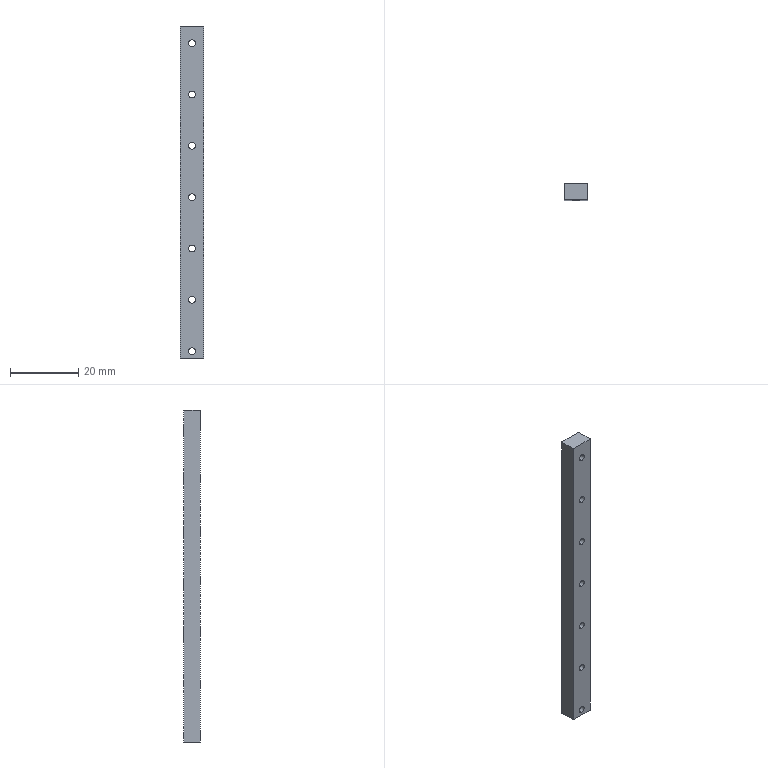Part | SolidWorks | features ICE 2, Extrusion 1, LPattern 1 | 1 solid | 41 faces | box 7 x 4.8 x 97 mm | volume 2868 mm3 | cylinder 28 | plane 13 | commonest cylinder face diameters 2 x14 5 x14
STEP:
#1=CARTESIAN_POINT('',(0.,0.1503,4.5));
#2=VERTEX_POINT('',#1);
#3=CARTESIAN_POINT('',(1.5,0.1503,0.));
#4=VERTEX_POINT('',#3);
#5=CARTESIAN_POINT('',(0.,0.1503,2.));
#6=DIRECTION('',(0.,1.,0.));
#7=DIRECTION('',(0.,0.,1.));
#8=AXIS2_PLACEMENT_3D('',#5,#6,#7);
#9=CIRCLE('',#8,2.5);
#10=EDGE_CURVE('',#2,#4,#9,.T.);
#11=ORIENTED_EDGE('',*,*,#10,.F.);
#12=CARTESIAN_POINT('',(0.,2.65,4.5));
#13=VERTEX_POINT('',#12);
#14=CARTESIAN_POINT('',(0.,0.1503,4.5));
#15=DIRECTION('',(0.,1.,0.));
#16=VECTOR('',#15,1000.);
#17=LINE('',#14,#16);
#18=EDGE_CURVE('',#2,#13,#17,.T.);
#19=ORIENTED_EDGE('',*,*,#18,.T.);
#20=CARTESIAN_POINT('',(1.5,2.65,0.));
#21=VERTEX_POINT('',#20);
#22=CARTESIAN_POINT('',(0.,2.65,2.));
#23=DIRECTION('',(0.,1.,0.));
#24=DIRECTION('',(0.,0.,1.));
#25=AXIS2_PLACEMENT_3D('',#22,#23,#24);
#26=CIRCLE('',#25,2.5);
#27=EDGE_CURVE('',#13,#21,#26,.T.);
#28=ORIENTED_EDGE('',*,*,#27,.T.);
#29=CARTESIAN_POINT('',(1.5,0.1503,0.));
#30=DIRECTION('',(0.,1.,0.));
#31=VECTOR('',#30,1000.);
#32=LINE('',#29,#31);
#33=EDGE_CURVE('',#4,#21,#32,.T.);
#34=ORIENTED_EDGE('',*,*,#33,.F.);
#35=EDGE_LOOP('',(#11,#19,#28,#34));
#36=FACE_OUTER_BOUND('',#35,.T.);
#37=CARTESIAN_POINT('',(0.,0.1503,2.));
#38=DIRECTION('',(0.,1.,0.));
#39=DIRECTION('',(0.,0.,1.));
#40=AXIS2_PLACEMENT_3D('',#37,#38,#39);
#41=CYLINDRICAL_SURFACE('',#40,2.5);
#42=ADVANCED_FACE('',(#36),#41,.F.);
#43=CARTESIAN_POINT('',(0.,0.1503,14.5));
#44=VERTEX_POINT('',#43);
#45=CARTESIAN_POINT('',(0.,0.1503,19.5));
#46=VERTEX_POINT('',#45);
#47=CARTESIAN_POINT('',(0.,0.1503,17.));
#48=DIRECTION('',(0.,1.,0.));
#49=DIRECTION('',(0.,0.,1.));
#50=AXIS2_PLACEMENT_3D('',#47,#48,#49);
#51=CIRCLE('',#50,2.5);
#52=EDGE_CURVE('',#44,#46,#51,.T.);
#53=ORIENTED_EDGE('',*,*,#52,.F.);
#54=CARTESIAN_POINT('',(0.,2.65,14.5));
#55=VERTEX_POINT('',#54);
#56=CARTESIAN_POINT('',(0.,0.1503,14.5));
#57=DIRECTION('',(0.,1.,0.));
#58=VECTOR('',#57,1000.);
#59=LINE('',#56,#58);
#60=EDGE_CURVE('',#44,#55,#59,.T.);
#61=ORIENTED_EDGE('',*,*,#60,.T.);
#62=CARTESIAN_POINT('',(0.,2.65,19.5));
#63=VERTEX_POINT('',#62);
#64=CARTESIAN_POINT('',(0.,2.65,17.));
#65=DIRECTION('',(0.,1.,0.));
#66=DIRECTION('',(0.,0.,1.));
#67=AXIS2_PLACEMENT_3D('',#64,#65,#66);
#68=CIRCLE('',#67,2.5);
#69=EDGE_CURVE('',#55,#63,#68,.T.);
#70=ORIENTED_EDGE('',*,*,#69,.T.);
#71=CARTESIAN_POINT('',(0.,0.1503,19.5));
#72=DIRECTION('',(0.,1.,0.));
#73=VECTOR('',#72,1000.);
#74=LINE('',#71,#73);
#75=EDGE_CURVE('',#46,#63,#74,.T.);
#76=ORIENTED_EDGE('',*,*,#75,.F.);
#77=EDGE_LOOP('',(#53,#61,#70,#76));
#78=FACE_OUTER_BOUND('',#77,.T.);
#79=CARTESIAN_POINT('',(0.,0.1503,17.));
#80=DIRECTION('',(0.,1.,0.));
#81=DIRECTION('',(0.,0.,1.));
#82=AXIS2_PLACEMENT_3D('',#79,#80,#81);
#83=CYLINDRICAL_SURFACE('',#82,2.5);
#84=ADVANCED_FACE('',(#78),#83,.F.);
#85=CARTESIAN_POINT('',(0.,0.1503,29.5));
#86=VERTEX_POINT('',#85);
#87=CARTESIAN_POINT('',(0.,0.1503,34.5));
#88=VERTEX_POINT('',#87);
#89=CARTESIAN_POINT('',(0.,0.1503,32.));
#90=DIRECTION('',(0.,1.,0.));
#91=DIRECTION('',(0.,0.,1.));
#92=AXIS2_PLACEMENT_3D('',#89,#90,#91);
#93=CIRCLE('',#92,2.5);
#94=EDGE_CURVE('',#86,#88,#93,.T.);
#95=ORIENTED_EDGE('',*,*,#94,.F.);
#96=CARTESIAN_POINT('',(0.,2.65,29.5));
#97=VERTEX_POINT('',#96);
#98=CARTESIAN_POINT('',(0.,0.1503,29.5));
#99=DIRECTION('',(0.,1.,0.));
#100=VECTOR('',#99,1000.);
#101=LINE('',#98,#100);
#102=EDGE_CURVE('',#86,#97,#101,.T.);
#103=ORIENTED_EDGE('',*,*,#102,.T.);
#104=CARTESIAN_POINT('',(0.,2.65,34.5));
#105=VERTEX_POINT('',#104);
#106=CARTESIAN_POINT('',(0.,2.65,32.));
#107=DIRECTION('',(0.,1.,0.));
#108=DIRECTION('',(0.,0.,1.));
#109=AXIS2_PLACEMENT_3D('',#106,#107,#108);
#110=CIRCLE('',#109,2.5);
#111=EDGE_CURVE('',#97,#105,#110,.T.);
#112=ORIENTED_EDGE('',*,*,#111,.T.);
#113=CARTESIAN_POINT('',(0.,0.1503,34.5));
#114=DIRECTION('',(0.,1.,0.));
#115=VECTOR('',#114,1000.);
#116=LINE('',#113,#115);
#117=EDGE_CURVE('',#88,#105,#116,.T.);
#118=ORIENTED_EDGE('',*,*,#117,.F.);
#119=EDGE_LOOP('',(#95,#103,#112,#118));
#120=FACE_OUTER_BOUND('',#119,.T.);
#121=CARTESIAN_POINT('',(0.,0.1503,32.));
#122=DIRECTION('',(0.,1.,0.));
#123=DIRECTION('',(0.,0.,1.));
#124=AXIS2_PLACEMENT_3D('',#121,#122,#123);
#125=CYLINDRICAL_SURFACE('',#124,2.5);
#126=ADVANCED_FACE('',(#120),#125,.F.);
#127=CARTESIAN_POINT('',(0.,0.1503,44.5));
#128=VERTEX_POINT('',#127);
#129=CARTESIAN_POINT('',(0.,0.1503,49.5));
#130=VERTEX_POINT('',#129);
#131=CARTESIAN_POINT('',(0.,0.1503,47.));
#132=DIRECTION('',(0.,1.,0.));
#133=DIRECTION('',(0.,0.,1.));
#134=AXIS2_PLACEMENT_3D('',#131,#132,#133);
#135=CIRCLE('',#134,2.5);
#136=EDGE_CURVE('',#128,#130,#135,.T.);
#137=ORIENTED_EDGE('',*,*,#136,.F.);
#138=CARTESIAN_POINT('',(0.,2.65,44.5));
#139=VERTEX_POINT('',#138);
#140=CARTESIAN_POINT('',(0.,0.1503,44.5));
#141=DIRECTION('',(0.,1.,0.));
#142=VECTOR('',#141,1000.);
#143=LINE('',#140,#142);
#144=EDGE_CURVE('',#128,#139,#143,.T.);
#145=ORIENTED_EDGE('',*,*,#144,.T.);
#146=CARTESIAN_POINT('',(0.,2.65,49.5));
#147=VERTEX_POINT('',#146);
#148=CARTESIAN_POINT('',(0.,2.65,47.));
#149=DIRECTION('',(0.,1.,0.));
#150=DIRECTION('',(0.,0.,1.));
#151=AXIS2_PLACEMENT_3D('',#148,#149,#150);
#152=CIRCLE('',#151,2.5);
#153=EDGE_CURVE('',#139,#147,#152,.T.);
#154=ORIENTED_EDGE('',*,*,#153,.T.);
#155=CARTESIAN_POINT('',(0.,0.1503,49.5));
#156=DIRECTION('',(0.,1.,0.));
#157=VECTOR('',#156,1000.);
#158=LINE('',#155,#157);
#159=EDGE_CURVE('',#130,#147,#158,.T.);
#160=ORIENTED_EDGE('',*,*,#159,.F.);
#161=EDGE_LOOP('',(#137,#145,#154,#160));
#162=FACE_OUTER_BOUND('',#161,.T.);
#163=CARTESIAN_POINT('',(0.,0.1503,47.));
#164=DIRECTION('',(0.,1.,0.));
#165=DIRECTION('',(0.,0.,1.));
#166=AXIS2_PLACEMENT_3D('',#163,#164,#165);
#167=CYLINDRICAL_SURFACE('',#166,2.5);
#168=ADVANCED_FACE('',(#162),#167,.F.);
#169=CARTESIAN_POINT('',(0.,0.1503,59.5));
#170=VERTEX_POINT('',#169);
#171=CARTESIAN_POINT('',(0.,0.1503,64.5));
#172=VERTEX_POINT('',#171);
#173=CARTESIAN_POINT('',(0.,0.1503,62.));
#174=DIRECTION('',(0.,1.,0.));
#175=DIRECTION('',(0.,0.,1.));
#176=AXIS2_PLACEMENT_3D('',#173,#174,#175);
#177=CIRCLE('',#176,2.5);
#178=EDGE_CURVE('',#170,#172,#177,.T.);
#179=ORIENTED_EDGE('',*,*,#178,.F.);
#180=CARTESIAN_POINT('',(0.,2.65,59.5));
#181=VERTEX_POINT('',#180);
#182=CARTESIAN_POINT('',(0.,0.1503,59.5));
#183=DIRECTION('',(0.,1.,0.));
#184=VECTOR('',#183,1000.);
#185=LINE('',#182,#184);
#186=EDGE_CURVE('',#170,#181,#185,.T.);
#187=ORIENTED_EDGE('',*,*,#186,.T.);
#188=CARTESIAN_POINT('',(0.,2.65,64.5));
#189=VERTEX_POINT('',#188);
#190=CARTESIAN_POINT('',(0.,2.65,62.));
#191=DIRECTION('',(0.,1.,0.));
#192=DIRECTION('',(0.,0.,1.));
#193=AXIS2_PLACEMENT_3D('',#190,#191,#192);
#194=CIRCLE('',#193,2.5);
#195=EDGE_CURVE('',#181,#189,#194,.T.);
#196=ORIENTED_EDGE('',*,*,#195,.T.);
#197=CARTESIAN_POINT('',(0.,0.1503,64.5));
#198=DIRECTION('',(0.,1.,0.));
#199=VECTOR('',#198,1000.);
#200=LINE('',#197,#199);
#201=EDGE_CURVE('',#172,#189,#200,.T.);
#202=ORIENTED_EDGE('',*,*,#201,.F.);
#203=EDGE_LOOP('',(#179,#187,#196,#202));
#204=FACE_OUTER_BOUND('',#203,.T.);
#205=CARTESIAN_POINT('',(0.,0.1503,62.));
#206=DIRECTION('',(0.,1.,0.));
#207=DIRECTION('',(0.,0.,1.));
#208=AXIS2_PLACEMENT_3D('',#205,#206,#207);
#209=CYLINDRICAL_SURFACE('',#208,2.5);
#210=ADVANCED_FACE('',(#204),#209,.F.);
#211=CARTESIAN_POINT('',(0.,0.1503,74.5));
#212=VERTEX_POINT('',#211);
#213=CARTESIAN_POINT('',(0.,0.1503,79.5));
#214=VERTEX_POINT('',#213);
#215=CARTESIAN_POINT('',(0.,0.1503,77.));
#216=DIRECTION('',(0.,1.,0.));
#217=DIRECTION('',(0.,0.,1.));
#218=AXIS2_PLACEMENT_3D('',#215,#216,#217);
#219=CIRCLE('',#218,2.5);
#220=EDGE_CURVE('',#212,#214,#219,.T.);
#221=ORIENTED_EDGE('',*,*,#220,.F.);
#222=CARTESIAN_POINT('',(0.,2.65,74.5));
#223=VERTEX_POINT('',#222);
#224=CARTESIAN_POINT('',(0.,0.1503,74.5));
#225=DIRECTION('',(0.,1.,0.));
#226=VECTOR('',#225,1000.);
#227=LINE('',#224,#226);
#228=EDGE_CURVE('',#212,#223,#227,.T.);
#229=ORIENTED_EDGE('',*,*,#228,.T.);
#230=CARTESIAN_POINT('',(0.,2.65,79.5));
#231=VERTEX_POINT('',#230);
#232=CARTESIAN_POINT('',(0.,2.65,77.));
#233=DIRECTION('',(0.,1.,0.));
#234=DIRECTION('',(0.,0.,1.));
#235=AXIS2_PLACEMENT_3D('',#232,#233,#234);
#236=CIRCLE('',#235,2.5);
#237=EDGE_CURVE('',#223,#231,#236,.T.);
#238=ORIENTED_EDGE('',*,*,#237,.T.);
#239=CARTESIAN_POINT('',(0.,0.1503,79.5));
#240=DIRECTION('',(0.,1.,0.));
#241=VECTOR('',#240,1000.);
#242=LINE('',#239,#241);
#243=EDGE_CURVE('',#214,#231,#242,.T.);
#244=ORIENTED_EDGE('',*,*,#243,.F.);
#245=EDGE_LOOP('',(#221,#229,#238,#244));
#246=FACE_OUTER_BOUND('',#245,.T.);
#247=CARTESIAN_POINT('',(0.,0.1503,77.));
#248=DIRECTION('',(0.,1.,0.));
#249=DIRECTION('',(0.,0.,1.));
#250=AXIS2_PLACEMENT_3D('',#247,#248,#249);
#251=CYLINDRICAL_SURFACE('',#250,2.5);
#252=ADVANCED_FACE('',(#246),#251,.F.);
#253=CARTESIAN_POINT('',(0.,0.1503,89.5));
#254=VERTEX_POINT('',#253);
#255=CARTESIAN_POINT('',(0.,0.1503,94.5));
#256=VERTEX_POINT('',#255);
#257=CARTESIAN_POINT('',(0.,0.1503,92.));
#258=DIRECTION('',(0.,1.,0.));
#259=DIRECTION('',(0.,0.,1.));
#260=AXIS2_PLACEMENT_3D('',#257,#258,#259);
#261=CIRCLE('',#260,2.5);
#262=EDGE_CURVE('',#254,#256,#261,.T.);
#263=ORIENTED_EDGE('',*,*,#262,.F.);
#264=CARTESIAN_POINT('',(0.,2.65,89.5));
#265=VERTEX_POINT('',#264);
#266=CARTESIAN_POINT('',(0.,0.1503,89.5));
#267=DIRECTION('',(0.,1.,0.));
#268=VECTOR('',#267,1000.);
#269=LINE('',#266,#268);
#270=EDGE_CURVE('',#254,#265,#269,.T.);
#271=ORIENTED_EDGE('',*,*,#270,.T.);
#272=CARTESIAN_POINT('',(0.,2.65,94.5));
#273=VERTEX_POINT('',#272);
#274=CARTESIAN_POINT('',(0.,2.65,92.));
#275=DIRECTION('',(0.,1.,0.));
#276=DIRECTION('',(0.,0.,1.));
#277=AXIS2_PLACEMENT_3D('',#274,#275,#276);
#278=CIRCLE('',#277,2.5);
#279=EDGE_CURVE('',#265,#273,#278,.T.);
#280=ORIENTED_EDGE('',*,*,#279,.T.);
#281=CARTESIAN_POINT('',(0.,0.1503,94.5));
#282=DIRECTION('',(0.,1.,0.));
#283=VECTOR('',#282,1000.);
#284=LINE('',#281,#283);
#285=EDGE_CURVE('',#256,#273,#284,.T.);
#286=ORIENTED_EDGE('',*,*,#285,.F.);
#287=EDGE_LOOP('',(#263,#271,#280,#286));
#288=FACE_OUTER_BOUND('',#287,.T.);
#289=CARTESIAN_POINT('',(0.,0.1503,92.));
#290=DIRECTION('',(0.,1.,0.));
#291=DIRECTION('',(0.,0.,1.));
#292=AXIS2_PLACEMENT_3D('',#289,#290,#291);
#293=CYLINDRICAL_SURFACE('',#292,2.5);
#294=ADVANCED_FACE('',(#288),#293,.F.);
#295=CARTESIAN_POINT('',(0.,-2.15,91.));
#296=VERTEX_POINT('',#295);
#297=CARTESIAN_POINT('',(0.,-2.15,93.));
#298=VERTEX_POINT('',#297);
#299=CARTESIAN_POINT('',(0.,-2.15,92.));
#300=DIRECTION('',(0.,1.,0.));
#301=DIRECTION('',(0.,0.,1.));
#302=AXIS2_PLACEMENT_3D('',#299,#300,#301);
#303=CIRCLE('',#302,1.);
#304=EDGE_CURVE('',#296,#298,#303,.T.);
#305=ORIENTED_EDGE('',*,*,#304,.F.);
#306=CARTESIAN_POINT('',(0.,0.1503,91.));
#307=VERTEX_POINT('',#306);
#308=CARTESIAN_POINT('',(0.,-665.35,91.));
#309=DIRECTION('',(0.,1.,0.));
#310=VECTOR('',#309,1000.);
#311=LINE('',#308,#310);
#312=EDGE_CURVE('',#296,#307,#311,.T.);
#313=ORIENTED_EDGE('',*,*,#312,.T.);
#314=CARTESIAN_POINT('',(0.,0.1503,93.));
#315=VERTEX_POINT('',#314);
#316=CARTESIAN_POINT('',(0.,0.1503,92.));
#317=DIRECTION('',(0.,-1.,0.));
#318=DIRECTION('',(0.,0.,1.));
#319=AXIS2_PLACEMENT_3D('',#316,#317,#318);
#320=CIRCLE('',#319,1.);
#321=EDGE_CURVE('',#315,#307,#320,.T.);
#322=ORIENTED_EDGE('',*,*,#321,.F.);
#323=CARTESIAN_POINT('',(0.,-665.35,93.));
#324=DIRECTION('',(0.,1.,0.));
#325=VECTOR('',#324,1000.);
#326=LINE('',#323,#325);
#327=EDGE_CURVE('',#298,#315,#326,.T.);
#328=ORIENTED_EDGE('',*,*,#327,.F.);
#329=EDGE_LOOP('',(#305,#313,#322,#328));
#330=FACE_OUTER_BOUND('',#329,.T.);
#331=CARTESIAN_POINT('',(0.,-665.35,92.));
#332=DIRECTION('',(0.,1.,0.));
#333=DIRECTION('',(0.,0.,1.));
#334=AXIS2_PLACEMENT_3D('',#331,#332,#333);
#335=CYLINDRICAL_SURFACE('',#334,1.);
#336=ADVANCED_FACE('',(#330),#335,.F.);
#337=CARTESIAN_POINT('',(0.,-2.15,76.));
#338=VERTEX_POINT('',#337);
#339=CARTESIAN_POINT('',(0.,-2.15,78.));
#340=VERTEX_POINT('',#339);
#341=CARTESIAN_POINT('',(0.,-2.15,77.));
#342=DIRECTION('',(0.,1.,0.));
#343=DIRECTION('',(0.,0.,1.));
#344=AXIS2_PLACEMENT_3D('',#341,#342,#343);
#345=CIRCLE('',#344,1.);
#346=EDGE_CURVE('',#338,#340,#345,.T.);
#347=ORIENTED_EDGE('',*,*,#346,.F.);
#348=CARTESIAN_POINT('',(0.,0.1503,76.));
#349=VERTEX_POINT('',#348);
#350=CARTESIAN_POINT('',(0.,-665.35,76.));
#351=DIRECTION('',(0.,1.,0.));
#352=VECTOR('',#351,1000.);
#353=LINE('',#350,#352);
#354=EDGE_CURVE('',#338,#349,#353,.T.);
#355=ORIENTED_EDGE('',*,*,#354,.T.);
#356=CARTESIAN_POINT('',(0.,0.1503,78.));
#357=VERTEX_POINT('',#356);
#358=CARTESIAN_POINT('',(0.,0.1503,77.));
#359=DIRECTION('',(0.,-1.,0.));
#360=DIRECTION('',(0.,0.,1.));
#361=AXIS2_PLACEMENT_3D('',#358,#359,#360);
#362=CIRCLE('',#361,1.);
#363=EDGE_CURVE('',#357,#349,#362,.T.);
#364=ORIENTED_EDGE('',*,*,#363,.F.);
#365=CARTESIAN_POINT('',(0.,-665.35,78.));
#366=DIRECTION('',(0.,1.,0.));
#367=VECTOR('',#366,1000.);
#368=LINE('',#365,#367);
#369=EDGE_CURVE('',#340,#357,#368,.T.);
#370=ORIENTED_EDGE('',*,*,#369,.F.);
#371=EDGE_LOOP('',(#347,#355,#364,#370));
#372=FACE_OUTER_BOUND('',#371,.T.);
#373=CARTESIAN_POINT('',(0.,-665.35,77.));
#374=DIRECTION('',(0.,1.,0.));
#375=DIRECTION('',(0.,0.,1.));
#376=AXIS2_PLACEMENT_3D('',#373,#374,#375);
#377=CYLINDRICAL_SURFACE('',#376,1.);
#378=ADVANCED_FACE('',(#372),#377,.F.);
#379=CARTESIAN_POINT('',(0.,-2.15,61.));
#380=VERTEX_POINT('',#379);
#381=CARTESIAN_POINT('',(0.,-2.15,63.));
#382=VERTEX_POINT('',#381);
#383=CARTESIAN_POINT('',(0.,-2.15,62.));
#384=DIRECTION('',(0.,1.,0.));
#385=DIRECTION('',(0.,0.,1.));
#386=AXIS2_PLACEMENT_3D('',#383,#384,#385);
#387=CIRCLE('',#386,1.);
#388=EDGE_CURVE('',#380,#382,#387,.T.);
#389=ORIENTED_EDGE('',*,*,#388,.F.);
#390=CARTESIAN_POINT('',(0.,0.1503,61.));
#391=VERTEX_POINT('',#390);
#392=CARTESIAN_POINT('',(0.,-665.35,61.));
#393=DIRECTION('',(0.,1.,0.));
#394=VECTOR('',#393,1000.);
#395=LINE('',#392,#394);
#396=EDGE_CURVE('',#380,#391,#395,.T.);
#397=ORIENTED_EDGE('',*,*,#396,.T.);
#398=CARTESIAN_POINT('',(0.,0.1503,63.));
#399=VERTEX_POINT('',#398);
#400=CARTESIAN_POINT('',(0.,0.1503,62.));
#401=DIRECTION('',(0.,-1.,0.));
#402=DIRECTION('',(0.,0.,1.));
#403=AXIS2_PLACEMENT_3D('',#400,#401,#402);
#404=CIRCLE('',#403,1.);
#405=EDGE_CURVE('',#399,#391,#404,.T.);
#406=ORIENTED_EDGE('',*,*,#405,.F.);
#407=CARTESIAN_POINT('',(0.,-665.35,63.));
#408=DIRECTION('',(0.,1.,0.));
#409=VECTOR('',#408,1000.);
#410=LINE('',#407,#409);
#411=EDGE_CURVE('',#382,#399,#410,.T.);
#412=ORIENTED_EDGE('',*,*,#411,.F.);
#413=EDGE_LOOP('',(#389,#397,#406,#412));
#414=FACE_OUTER_BOUND('',#413,.T.);
#415=CARTESIAN_POINT('',(0.,-665.35,62.));
#416=DIRECTION('',(0.,1.,0.));
#417=DIRECTION('',(0.,0.,1.));
#418=AXIS2_PLACEMENT_3D('',#415,#416,#417);
#419=CYLINDRICAL_SURFACE('',#418,1.);
#420=ADVANCED_FACE('',(#414),#419,.F.);
#421=CARTESIAN_POINT('',(0.,-2.15,46.));
#422=VERTEX_POINT('',#421);
#423=CARTESIAN_POINT('',(0.,-2.15,48.));
#424=VERTEX_POINT('',#423);
#425=CARTESIAN_POINT('',(0.,-2.15,47.));
#426=DIRECTION('',(0.,1.,0.));
#427=DIRECTION('',(0.,0.,1.));
#428=AXIS2_PLACEMENT_3D('',#425,#426,#427);
#429=CIRCLE('',#428,1.);
#430=EDGE_CURVE('',#422,#424,#429,.T.);
#431=ORIENTED_EDGE('',*,*,#430,.F.);
#432=CARTESIAN_POINT('',(0.,0.1503,46.));
#433=VERTEX_POINT('',#432);
#434=CARTESIAN_POINT('',(0.,-665.35,46.));
#435=DIRECTION('',(0.,1.,0.));
#436=VECTOR('',#435,1000.);
#437=LINE('',#434,#436);
#438=EDGE_CURVE('',#422,#433,#437,.T.);
#439=ORIENTED_EDGE('',*,*,#438,.T.);
#440=CARTESIAN_POINT('',(0.,0.1503,48.));
#441=VERTEX_POINT('',#440);
#442=CARTESIAN_POINT('',(0.,0.1503,47.));
#443=DIRECTION('',(0.,-1.,0.));
#444=DIRECTION('',(0.,0.,1.));
#445=AXIS2_PLACEMENT_3D('',#442,#443,#444);
#446=CIRCLE('',#445,1.);
#447=EDGE_CURVE('',#441,#433,#446,.T.);
#448=ORIENTED_EDGE('',*,*,#447,.F.);
#449=CARTESIAN_POINT('',(0.,-665.35,48.));
#450=DIRECTION('',(0.,1.,0.));
#451=VECTOR('',#450,1000.);
#452=LINE('',#449,#451);
#453=EDGE_CURVE('',#424,#441,#452,.T.);
#454=ORIENTED_EDGE('',*,*,#453,.F.);
#455=EDGE_LOOP('',(#431,#439,#448,#454));
#456=FACE_OUTER_BOUND('',#455,.T.);
#457=CARTESIAN_POINT('',(0.,-665.35,47.));
#458=DIRECTION('',(0.,1.,0.));
#459=DIRECTION('',(0.,0.,1.));
#460=AXIS2_PLACEMENT_3D('',#457,#458,#459);
#461=CYLINDRICAL_SURFACE('',#460,1.);
#462=ADVANCED_FACE('',(#456),#461,.F.);
#463=CARTESIAN_POINT('',(0.,-2.15,31.));
#464=VERTEX_POINT('',#463);
#465=CARTESIAN_POINT('',(0.,-2.15,33.));
#466=VERTEX_POINT('',#465);
#467=CARTESIAN_POINT('',(0.,-2.15,32.));
#468=DIRECTION('',(0.,1.,0.));
#469=DIRECTION('',(0.,0.,1.));
#470=AXIS2_PLACEMENT_3D('',#467,#468,#469);
#471=CIRCLE('',#470,1.);
#472=EDGE_CURVE('',#464,#466,#471,.T.);
#473=ORIENTED_EDGE('',*,*,#472,.F.);
#474=CARTESIAN_POINT('',(0.,0.1503,31.));
#475=VERTEX_POINT('',#474);
#476=CARTESIAN_POINT('',(0.,-665.35,31.));
#477=DIRECTION('',(0.,1.,0.));
#478=VECTOR('',#477,1000.);
#479=LINE('',#476,#478);
#480=EDGE_CURVE('',#464,#475,#479,.T.);
#481=ORIENTED_EDGE('',*,*,#480,.T.);
#482=CARTESIAN_POINT('',(0.,0.1503,33.));
#483=VERTEX_POINT('',#482);
#484=CARTESIAN_POINT('',(0.,0.1503,32.));
#485=DIRECTION('',(0.,-1.,0.));
#486=DIRECTION('',(0.,0.,1.));
#487=AXIS2_PLACEMENT_3D('',#484,#485,#486);
#488=CIRCLE('',#487,1.);
#489=EDGE_CURVE('',#483,#475,#488,.T.);
#490=ORIENTED_EDGE('',*,*,#489,.F.);
#491=CARTESIAN_POINT('',(0.,-665.35,33.));
#492=DIRECTION('',(0.,1.,0.));
#493=VECTOR('',#492,1000.);
#494=LINE('',#491,#493);
#495=EDGE_CURVE('',#466,#483,#494,.T.);
#496=ORIENTED_EDGE('',*,*,#495,.F.);
#497=EDGE_LOOP('',(#473,#481,#490,#496));
#498=FACE_OUTER_BOUND('',#497,.T.);
#499=CARTESIAN_POINT('',(0.,-665.35,32.));
#500=DIRECTION('',(0.,1.,0.));
#501=DIRECTION('',(0.,0.,1.));
#502=AXIS2_PLACEMENT_3D('',#499,#500,#501);
#503=CYLINDRICAL_SURFACE('',#502,1.);
#504=ADVANCED_FACE('',(#498),#503,.F.);
#505=CARTESIAN_POINT('',(0.,-2.15,16.));
#506=VERTEX_POINT('',#505);
#507=CARTESIAN_POINT('',(0.,-2.15,18.));
#508=VERTEX_POINT('',#507);
#509=CARTESIAN_POINT('',(0.,-2.15,17.));
#510=DIRECTION('',(0.,1.,0.));
#511=DIRECTION('',(0.,0.,1.));
#512=AXIS2_PLACEMENT_3D('',#509,#510,#511);
#513=CIRCLE('',#512,1.);
#514=EDGE_CURVE('',#506,#508,#513,.T.);
#515=ORIENTED_EDGE('',*,*,#514,.F.);
#516=CARTESIAN_POINT('',(0.,0.1503,16.));
#517=VERTEX_POINT('',#516);
#518=CARTESIAN_POINT('',(0.,-665.35,16.));
#519=DIRECTION('',(0.,1.,0.));
#520=VECTOR('',#519,1000.);
#521=LINE('',#518,#520);
#522=EDGE_CURVE('',#506,#517,#521,.T.);
#523=ORIENTED_EDGE('',*,*,#522,.T.);
#524=CARTESIAN_POINT('',(0.,0.1503,18.));
#525=VERTEX_POINT('',#524);
#526=CARTESIAN_POINT('',(0.,0.1503,17.));
#527=DIRECTION('',(0.,-1.,0.));
#528=DIRECTION('',(0.,0.,1.));
#529=AXIS2_PLACEMENT_3D('',#526,#527,#528);
#530=CIRCLE('',#529,1.);
#531=EDGE_CURVE('',#525,#517,#530,.T.);
#532=ORIENTED_EDGE('',*,*,#531,.F.);
#533=CARTESIAN_POINT('',(0.,-665.35,18.));
#534=DIRECTION('',(0.,1.,0.));
#535=VECTOR('',#534,1000.);
#536=LINE('',#533,#535);
#537=EDGE_CURVE('',#508,#525,#536,.T.);
#538=ORIENTED_EDGE('',*,*,#537,.F.);
#539=EDGE_LOOP('',(#515,#523,#532,#538));
#540=FACE_OUTER_BOUND('',#539,.T.);
#541=CARTESIAN_POINT('',(0.,-665.35,17.));
#542=DIRECTION('',(0.,1.,0.));
#543=DIRECTION('',(0.,0.,1.));
#544=AXIS2_PLACEMENT_3D('',#541,#542,#543);
#545=CYLINDRICAL_SURFACE('',#544,1.);
#546=ADVANCED_FACE('',(#540),#545,.F.);
#547=CARTESIAN_POINT('',(0.,-2.15,1.));
#548=VERTEX_POINT('',#547);
#549=CARTESIAN_POINT('',(0.,-2.15,3.));
#550=VERTEX_POINT('',#549);
#551=CARTESIAN_POINT('',(0.,-2.15,2.));
#552=DIRECTION('',(0.,1.,0.));
#553=DIRECTION('',(0.,0.,1.));
#554=AXIS2_PLACEMENT_3D('',#551,#552,#553);
#555=CIRCLE('',#554,1.);
#556=EDGE_CURVE('',#548,#550,#555,.T.);
#557=ORIENTED_EDGE('',*,*,#556,.F.);
#558=CARTESIAN_POINT('',(0.,0.1503,1.));
#559=VERTEX_POINT('',#558);
#560=CARTESIAN_POINT('',(0.,-665.35,1.));
#561=DIRECTION('',(0.,1.,0.));
#562=VECTOR('',#561,1000.);
#563=LINE('',#560,#562);
#564=EDGE_CURVE('',#548,#559,#563,.T.);
#565=ORIENTED_EDGE('',*,*,#564,.T.);
#566=CARTESIAN_POINT('',(0.,0.1503,3.));
#567=VERTEX_POINT('',#566);
#568=CARTESIAN_POINT('',(0.,0.1503,2.));
#569=DIRECTION('',(0.,-1.,0.));
#570=DIRECTION('',(0.,0.,1.));
#571=AXIS2_PLACEMENT_3D('',#568,#569,#570);
#572=CIRCLE('',#571,1.);
#573=EDGE_CURVE('',#567,#559,#572,.T.);
#574=ORIENTED_EDGE('',*,*,#573,.F.);
#575=CARTESIAN_POINT('',(0.,-665.35,3.));
#576=DIRECTION('',(0.,1.,0.));
#577=VECTOR('',#576,1000.);
#578=LINE('',#575,#577);
#579=EDGE_CURVE('',#550,#567,#578,.T.);
#580=ORIENTED_EDGE('',*,*,#579,.F.);
#581=EDGE_LOOP('',(#557,#565,#574,#580));
#582=FACE_OUTER_BOUND('',#581,.T.);
#583=CARTESIAN_POINT('',(0.,-665.35,2.));
#584=DIRECTION('',(0.,1.,0.));
#585=DIRECTION('',(0.,0.,1.));
#586=AXIS2_PLACEMENT_3D('',#583,#584,#585);
#587=CYLINDRICAL_SURFACE('',#586,1.);
#588=ADVANCED_FACE('',(#582),#587,.F.);
#589=ORIENTED_EDGE('',*,*,#564,.F.);
#590=CARTESIAN_POINT('',(0.,-2.15,2.));
#591=DIRECTION('',(0.,1.,0.));
#592=DIRECTION('',(0.,0.,1.));
#593=AXIS2_PLACEMENT_3D('',#590,#591,#592);
#594=CIRCLE('',#593,1.);
#595=EDGE_CURVE('',#550,#548,#594,.T.);
#596=ORIENTED_EDGE('',*,*,#595,.F.);
#597=ORIENTED_EDGE('',*,*,#579,.T.);
#598=CARTESIAN_POINT('',(0.,0.1503,2.));
#599=DIRECTION('',(0.,-1.,0.));
#600=DIRECTION('',(0.,0.,1.));
#601=AXIS2_PLACEMENT_3D('',#598,#599,#600);
#602=CIRCLE('',#601,1.);
#603=EDGE_CURVE('',#559,#567,#602,.T.);
#604=ORIENTED_EDGE('',*,*,#603,.F.);
#605=EDGE_LOOP('',(#589,#596,#597,#604));
#606=FACE_OUTER_BOUND('',#605,.T.);
#607=CARTESIAN_POINT('',(0.,-665.35,2.));
#608=DIRECTION('',(0.,1.,0.));
#609=DIRECTION('',(0.,0.,1.));
#610=AXIS2_PLACEMENT_3D('',#607,#608,#609);
#611=CYLINDRICAL_SURFACE('',#610,1.);
#612=ADVANCED_FACE('',(#606),#611,.F.);
#613=ORIENTED_EDGE('',*,*,#522,.F.);
#614=CARTESIAN_POINT('',(0.,-2.15,17.));
#615=DIRECTION('',(0.,1.,0.));
#616=DIRECTION('',(0.,0.,1.));
#617=AXIS2_PLACEMENT_3D('',#614,#615,#616);
#618=CIRCLE('',#617,1.);
#619=EDGE_CURVE('',#508,#506,#618,.T.);
#620=ORIENTED_EDGE('',*,*,#619,.F.);
#621=ORIENTED_EDGE('',*,*,#537,.T.);
#622=CARTESIAN_POINT('',(0.,0.1503,17.));
#623=DIRECTION('',(0.,-1.,0.));
#624=DIRECTION('',(0.,0.,1.));
#625=AXIS2_PLACEMENT_3D('',#622,#623,#624);
#626=CIRCLE('',#625,1.);
#627=EDGE_CURVE('',#517,#525,#626,.T.);
#628=ORIENTED_EDGE('',*,*,#627,.F.);
#629=EDGE_LOOP('',(#613,#620,#621,#628));
#630=FACE_OUTER_BOUND('',#629,.T.);
#631=CARTESIAN_POINT('',(0.,-665.35,17.));
#632=DIRECTION('',(0.,1.,0.));
#633=DIRECTION('',(0.,0.,1.));
#634=AXIS2_PLACEMENT_3D('',#631,#632,#633);
#635=CYLINDRICAL_SURFACE('',#634,1.);
#636=ADVANCED_FACE('',(#630),#635,.F.);
#637=ORIENTED_EDGE('',*,*,#480,.F.);
#638=CARTESIAN_POINT('',(0.,-2.15,32.));
#639=DIRECTION('',(0.,1.,0.));
#640=DIRECTION('',(0.,0.,1.));
#641=AXIS2_PLACEMENT_3D('',#638,#639,#640);
#642=CIRCLE('',#641,1.);
#643=EDGE_CURVE('',#466,#464,#642,.T.);
#644=ORIENTED_EDGE('',*,*,#643,.F.);
#645=ORIENTED_EDGE('',*,*,#495,.T.);
#646=CARTESIAN_POINT('',(0.,0.1503,32.));
#647=DIRECTION('',(0.,-1.,0.));
#648=DIRECTION('',(0.,0.,1.));
#649=AXIS2_PLACEMENT_3D('',#646,#647,#648);
#650=CIRCLE('',#649,1.);
#651=EDGE_CURVE('',#475,#483,#650,.T.);
#652=ORIENTED_EDGE('',*,*,#651,.F.);
#653=EDGE_LOOP('',(#637,#644,#645,#652));
#654=FACE_OUTER_BOUND('',#653,.T.);
#655=CARTESIAN_POINT('',(0.,-665.35,32.));
#656=DIRECTION('',(0.,1.,0.));
#657=DIRECTION('',(0.,0.,1.));
#658=AXIS2_PLACEMENT_3D('',#655,#656,#657);
#659=CYLINDRICAL_SURFACE('',#658,1.);
#660=ADVANCED_FACE('',(#654),#659,.F.);
#661=ORIENTED_EDGE('',*,*,#438,.F.);
#662=CARTESIAN_POINT('',(0.,-2.15,47.));
#663=DIRECTION('',(0.,1.,0.));
#664=DIRECTION('',(0.,0.,1.));
#665=AXIS2_PLACEMENT_3D('',#662,#663,#664);
#666=CIRCLE('',#665,1.);
#667=EDGE_CURVE('',#424,#422,#666,.T.);
#668=ORIENTED_EDGE('',*,*,#667,.F.);
#669=ORIENTED_EDGE('',*,*,#453,.T.);
#670=CARTESIAN_POINT('',(0.,0.1503,47.));
#671=DIRECTION('',(0.,-1.,0.));
#672=DIRECTION('',(0.,0.,1.));
#673=AXIS2_PLACEMENT_3D('',#670,#671,#672);
#674=CIRCLE('',#673,1.);
#675=EDGE_CURVE('',#433,#441,#674,.T.);
#676=ORIENTED_EDGE('',*,*,#675,.F.);
#677=EDGE_LOOP('',(#661,#668,#669,#676));
#678=FACE_OUTER_BOUND('',#677,.T.);
#679=CARTESIAN_POINT('',(0.,-665.35,47.));
#680=DIRECTION('',(0.,1.,0.));
#681=DIRECTION('',(0.,0.,1.));
#682=AXIS2_PLACEMENT_3D('',#679,#680,#681);
#683=CYLINDRICAL_SURFACE('',#682,1.);
#684=ADVANCED_FACE('',(#678),#683,.F.);
#685=ORIENTED_EDGE('',*,*,#396,.F.);
#686=CARTESIAN_POINT('',(0.,-2.15,62.));
#687=DIRECTION('',(0.,1.,0.));
#688=DIRECTION('',(0.,0.,1.));
#689=AXIS2_PLACEMENT_3D('',#686,#687,#688);
#690=CIRCLE('',#689,1.);
#691=EDGE_CURVE('',#382,#380,#690,.T.);
#692=ORIENTED_EDGE('',*,*,#691,.F.);
#693=ORIENTED_EDGE('',*,*,#411,.T.);
#694=CARTESIAN_POINT('',(0.,0.1503,62.));
#695=DIRECTION('',(0.,-1.,0.));
#696=DIRECTION('',(0.,0.,1.));
#697=AXIS2_PLACEMENT_3D('',#694,#695,#696);
#698=CIRCLE('',#697,1.);
#699=EDGE_CURVE('',#391,#399,#698,.T.);
#700=ORIENTED_EDGE('',*,*,#699,.F.);
#701=EDGE_LOOP('',(#685,#692,#693,#700));
#702=FACE_OUTER_BOUND('',#701,.T.);
#703=CARTESIAN_POINT('',(0.,-665.35,62.));
#704=DIRECTION('',(0.,1.,0.));
#705=DIRECTION('',(0.,0.,1.));
#706=AXIS2_PLACEMENT_3D('',#703,#704,#705);
#707=CYLINDRICAL_SURFACE('',#706,1.);
#708=ADVANCED_FACE('',(#702),#707,.F.);
#709=ORIENTED_EDGE('',*,*,#354,.F.);
#710=CARTESIAN_POINT('',(0.,-2.15,77.));
#711=DIRECTION('',(0.,1.,0.));
#712=DIRECTION('',(0.,0.,1.));
#713=AXIS2_PLACEMENT_3D('',#710,#711,#712);
#714=CIRCLE('',#713,1.);
#715=EDGE_CURVE('',#340,#338,#714,.T.);
#716=ORIENTED_EDGE('',*,*,#715,.F.);
#717=ORIENTED_EDGE('',*,*,#369,.T.);
#718=CARTESIAN_POINT('',(0.,0.1503,77.));
#719=DIRECTION('',(0.,-1.,0.));
#720=DIRECTION('',(0.,0.,1.));
#721=AXIS2_PLACEMENT_3D('',#718,#719,#720);
#722=CIRCLE('',#721,1.);
#723=EDGE_CURVE('',#349,#357,#722,.T.);
#724=ORIENTED_EDGE('',*,*,#723,.F.);
#725=EDGE_LOOP('',(#709,#716,#717,#724));
#726=FACE_OUTER_BOUND('',#725,.T.);
#727=CARTESIAN_POINT('',(0.,-665.35,77.));
#728=DIRECTION('',(0.,1.,0.));
#729=DIRECTION('',(0.,0.,1.));
#730=AXIS2_PLACEMENT_3D('',#727,#728,#729);
#731=CYLINDRICAL_SURFACE('',#730,1.);
#732=ADVANCED_FACE('',(#726),#731,.F.);
#733=ORIENTED_EDGE('',*,*,#312,.F.);
#734=CARTESIAN_POINT('',(0.,-2.15,92.));
#735=DIRECTION('',(0.,1.,0.));
#736=DIRECTION('',(0.,0.,1.));
#737=AXIS2_PLACEMENT_3D('',#734,#735,#736);
#738=CIRCLE('',#737,1.);
#739=EDGE_CURVE('',#298,#296,#738,.T.);
#740=ORIENTED_EDGE('',*,*,#739,.F.);
#741=ORIENTED_EDGE('',*,*,#327,.T.);
#742=CARTESIAN_POINT('',(0.,0.1503,92.));
#743=DIRECTION('',(0.,-1.,0.));
#744=DIRECTION('',(0.,0.,1.));
#745=AXIS2_PLACEMENT_3D('',#742,#743,#744);
#746=CIRCLE('',#745,1.);
#747=EDGE_CURVE('',#307,#315,#746,.T.);
#748=ORIENTED_EDGE('',*,*,#747,.F.);
#749=EDGE_LOOP('',(#733,#740,#741,#748));
#750=FACE_OUTER_BOUND('',#749,.T.);
#751=CARTESIAN_POINT('',(0.,-665.35,92.));
#752=DIRECTION('',(0.,1.,0.));
#753=DIRECTION('',(0.,0.,1.));
#754=AXIS2_PLACEMENT_3D('',#751,#752,#753);
#755=CYLINDRICAL_SURFACE('',#754,1.);
#756=ADVANCED_FACE('',(#750),#755,.F.);
#757=CARTESIAN_POINT('',(-3.5,2.65,0.));
#758=VERTEX_POINT('',#757);
#759=CARTESIAN_POINT('',(-3.5,-2.15,0.));
#760=VERTEX_POINT('',#759);
#761=CARTESIAN_POINT('',(-3.5,2.65,0.));
#762=DIRECTION('',(0.,-1.,0.));
#763=VECTOR('',#762,1000.);
#764=LINE('',#761,#763);
#765=EDGE_CURVE('',#758,#760,#764,.T.);
#766=ORIENTED_EDGE('',*,*,#765,.T.);
#767=CARTESIAN_POINT('',(-3.5,-2.15,97.));
#768=VERTEX_POINT('',#767);
#769=CARTESIAN_POINT('',(-3.5,-2.15,97.));
#770=DIRECTION('',(0.,0.,-1.));
#771=VECTOR('',#770,1000.);
#772=LINE('',#769,#771);
#773=EDGE_CURVE('',#768,#760,#772,.T.);
#774=ORIENTED_EDGE('',*,*,#773,.F.);
#775=CARTESIAN_POINT('',(-3.5,2.65,97.));
#776=VERTEX_POINT('',#775);
#777=CARTESIAN_POINT('',(-3.5,2.65,97.));
#778=DIRECTION('',(0.,-1.,0.));
#779=VECTOR('',#778,1000.);
#780=LINE('',#777,#779);
#781=EDGE_CURVE('',#776,#768,#780,.T.);
#782=ORIENTED_EDGE('',*,*,#781,.F.);
#783=CARTESIAN_POINT('',(-3.5,2.65,97.));
#784=DIRECTION('',(0.,0.,-1.));
#785=VECTOR('',#784,1000.);
#786=LINE('',#783,#785);
#787=EDGE_CURVE('',#776,#758,#786,.T.);
#788=ORIENTED_EDGE('',*,*,#787,.T.);
#789=EDGE_LOOP('',(#766,#774,#782,#788));
#790=FACE_OUTER_BOUND('',#789,.T.);
#791=CARTESIAN_POINT('',(-3.5,2.65,97.));
#792=DIRECTION('',(1.,0.,0.));
#793=DIRECTION('',(0.,0.,-1.));
#794=AXIS2_PLACEMENT_3D('',#791,#792,#793);
#795=PLANE('',#794);
#796=ADVANCED_FACE('',(#790),#795,.F.);
#797=ORIENTED_EDGE('',*,*,#715,.T.);
#798=ORIENTED_EDGE('',*,*,#346,.T.);
#799=EDGE_LOOP('',(#797,#798));
#800=FACE_BOUND('',#799,.T.);
#801=ORIENTED_EDGE('',*,*,#691,.T.);
#802=ORIENTED_EDGE('',*,*,#388,.T.);
#803=EDGE_LOOP('',(#801,#802));
#804=FACE_BOUND('',#803,.T.);
#805=ORIENTED_EDGE('',*,*,#667,.T.);
#806=ORIENTED_EDGE('',*,*,#430,.T.);
#807=EDGE_LOOP('',(#805,#806));
#808=FACE_BOUND('',#807,.T.);
#809=ORIENTED_EDGE('',*,*,#643,.T.);
#810=ORIENTED_EDGE('',*,*,#472,.T.);
#811=EDGE_LOOP('',(#809,#810));
#812=FACE_BOUND('',#811,.T.);
#813=ORIENTED_EDGE('',*,*,#619,.T.);
#814=ORIENTED_EDGE('',*,*,#514,.T.);
#815=EDGE_LOOP('',(#813,#814));
#816=FACE_BOUND('',#815,.T.);
#817=ORIENTED_EDGE('',*,*,#595,.T.);
#818=ORIENTED_EDGE('',*,*,#556,.T.);
#819=EDGE_LOOP('',(#817,#818));
#820=FACE_BOUND('',#819,.T.);
#821=ORIENTED_EDGE('',*,*,#739,.T.);
#822=ORIENTED_EDGE('',*,*,#304,.T.);
#823=EDGE_LOOP('',(#821,#822));
#824=FACE_BOUND('',#823,.T.);
#825=CARTESIAN_POINT('',(3.5,-2.15,0.));
#826=VERTEX_POINT('',#825);
#827=CARTESIAN_POINT('',(-3.5,-2.15,0.));
#828=DIRECTION('',(1.,0.,0.));
#829=VECTOR('',#828,1000.);
#830=LINE('',#827,#829);
#831=EDGE_CURVE('',#760,#826,#830,.T.);
#832=ORIENTED_EDGE('',*,*,#831,.T.);
#833=CARTESIAN_POINT('',(3.5,-2.15,97.));
#834=VERTEX_POINT('',#833);
#835=CARTESIAN_POINT('',(3.5,-2.15,97.));
#836=DIRECTION('',(0.,0.,-1.));
#837=VECTOR('',#836,1000.);
#838=LINE('',#835,#837);
#839=EDGE_CURVE('',#834,#826,#838,.T.);
#840=ORIENTED_EDGE('',*,*,#839,.F.);
#841=CARTESIAN_POINT('',(-3.5,-2.15,97.));
#842=DIRECTION('',(1.,0.,0.));
#843=VECTOR('',#842,1000.);
#844=LINE('',#841,#843);
#845=EDGE_CURVE('',#768,#834,#844,.T.);
#846=ORIENTED_EDGE('',*,*,#845,.F.);
#847=ORIENTED_EDGE('',*,*,#773,.T.);
#848=EDGE_LOOP('',(#832,#840,#846,#847));
#849=FACE_OUTER_BOUND('',#848,.T.);
#850=CARTESIAN_POINT('',(-3.5,-2.15,97.));
#851=DIRECTION('',(0.,1.,0.));
#852=DIRECTION('',(0.,0.,1.));
#853=AXIS2_PLACEMENT_3D('',#850,#851,#852);
#854=PLANE('',#853);
#855=ADVANCED_FACE('',(#800,#804,#808,#812,#816,#820,#824,#849),#854,.F.);
#856=CARTESIAN_POINT('',(3.5,2.65,0.));
#857=VERTEX_POINT('',#856);
#858=CARTESIAN_POINT('',(3.5,2.65,0.));
#859=DIRECTION('',(0.,-1.,0.));
#860=VECTOR('',#859,1000.);
#861=LINE('',#858,#860);
#862=EDGE_CURVE('',#857,#826,#861,.T.);
#863=ORIENTED_EDGE('',*,*,#862,.F.);
#864=CARTESIAN_POINT('',(3.5,2.65,97.));
#865=VERTEX_POINT('',#864);
#866=CARTESIAN_POINT('',(3.5,2.65,97.));
#867=DIRECTION('',(0.,0.,-1.));
#868=VECTOR('',#867,1000.);
#869=LINE('',#866,#868);
#870=EDGE_CURVE('',#865,#857,#869,.T.);
#871=ORIENTED_EDGE('',*,*,#870,.F.);
#872=CARTESIAN_POINT('',(3.5,2.65,97.));
#873=DIRECTION('',(0.,-1.,0.));
#874=VECTOR('',#873,1000.);
#875=LINE('',#872,#874);
#876=EDGE_CURVE('',#865,#834,#875,.T.);
#877=ORIENTED_EDGE('',*,*,#876,.T.);
#878=ORIENTED_EDGE('',*,*,#839,.T.);
#879=EDGE_LOOP('',(#863,#871,#877,#878));
#880=FACE_OUTER_BOUND('',#879,.T.);
#881=CARTESIAN_POINT('',(3.5,2.65,97.));
#882=DIRECTION('',(1.,0.,0.));
#883=DIRECTION('',(0.,1.,0.));
#884=AXIS2_PLACEMENT_3D('',#881,#882,#883);
#885=PLANE('',#884);
#886=ADVANCED_FACE('',(#880),#885,.T.);
#887=CARTESIAN_POINT('',(0.,2.65,77.));
#888=DIRECTION('',(0.,1.,0.));
#889=DIRECTION('',(0.,0.,1.));
#890=AXIS2_PLACEMENT_3D('',#887,#888,#889);
#891=CIRCLE('',#890,2.5);
#892=EDGE_CURVE('',#231,#223,#891,.T.);
#893=ORIENTED_EDGE('',*,*,#892,.F.);
#894=ORIENTED_EDGE('',*,*,#237,.F.);
#895=EDGE_LOOP('',(#893,#894));
#896=FACE_BOUND('',#895,.T.);
#897=CARTESIAN_POINT('',(0.,2.65,62.));
#898=DIRECTION('',(0.,1.,0.));
#899=DIRECTION('',(0.,0.,1.));
#900=AXIS2_PLACEMENT_3D('',#897,#898,#899);
#901=CIRCLE('',#900,2.5);
#902=EDGE_CURVE('',#189,#181,#901,.T.);
#903=ORIENTED_EDGE('',*,*,#902,.F.);
#904=ORIENTED_EDGE('',*,*,#195,.F.);
#905=EDGE_LOOP('',(#903,#904));
#906=FACE_BOUND('',#905,.T.);
#907=CARTESIAN_POINT('',(0.,2.65,47.));
#908=DIRECTION('',(0.,1.,0.));
#909=DIRECTION('',(0.,0.,1.));
#910=AXIS2_PLACEMENT_3D('',#907,#908,#909);
#911=CIRCLE('',#910,2.5);
#912=EDGE_CURVE('',#147,#139,#911,.T.);
#913=ORIENTED_EDGE('',*,*,#912,.F.);
#914=ORIENTED_EDGE('',*,*,#153,.F.);
#915=EDGE_LOOP('',(#913,#914));
#916=FACE_BOUND('',#915,.T.);
#917=CARTESIAN_POINT('',(0.,2.65,32.));
#918=DIRECTION('',(0.,1.,0.));
#919=DIRECTION('',(0.,0.,1.));
#920=AXIS2_PLACEMENT_3D('',#917,#918,#919);
#921=CIRCLE('',#920,2.5);
#922=EDGE_CURVE('',#105,#97,#921,.T.);
#923=ORIENTED_EDGE('',*,*,#922,.F.);
#924=ORIENTED_EDGE('',*,*,#111,.F.);
#925=EDGE_LOOP('',(#923,#924));
#926=FACE_BOUND('',#925,.T.);
#927=CARTESIAN_POINT('',(0.,2.65,17.));
#928=DIRECTION('',(0.,1.,0.));
#929=DIRECTION('',(0.,0.,1.));
#930=AXIS2_PLACEMENT_3D('',#927,#928,#929);
#931=CIRCLE('',#930,2.5);
#932=EDGE_CURVE('',#63,#55,#931,.T.);
#933=ORIENTED_EDGE('',*,*,#932,.F.);
#934=ORIENTED_EDGE('',*,*,#69,.F.);
#935=EDGE_LOOP('',(#933,#934));
#936=FACE_BOUND('',#935,.T.);
#937=CARTESIAN_POINT('',(-1.5,2.65,0.));
#938=VERTEX_POINT('',#937);
#939=CARTESIAN_POINT('',(0.,2.65,2.));
#940=DIRECTION('',(0.,1.,0.));
#941=DIRECTION('',(0.,0.,1.));
#942=AXIS2_PLACEMENT_3D('',#939,#940,#941);
#943=CIRCLE('',#942,2.5);
#944=EDGE_CURVE('',#938,#13,#943,.T.);
#945=ORIENTED_EDGE('',*,*,#944,.F.);
#946=CARTESIAN_POINT('',(-3.5,2.65,0.));
#947=DIRECTION('',(1.,0.,0.));
#948=VECTOR('',#947,1000.);
#949=LINE('',#946,#948);
#950=EDGE_CURVE('',#758,#938,#949,.T.);
#951=ORIENTED_EDGE('',*,*,#950,.F.);
#952=ORIENTED_EDGE('',*,*,#787,.F.);
#953=CARTESIAN_POINT('',(-3.5,2.65,97.));
#954=DIRECTION('',(1.,0.,0.));
#955=VECTOR('',#954,1000.);
#956=LINE('',#953,#955);
#957=EDGE_CURVE('',#776,#865,#956,.T.);
#958=ORIENTED_EDGE('',*,*,#957,.T.);
#959=ORIENTED_EDGE('',*,*,#870,.T.);
#960=CARTESIAN_POINT('',(-3.5,2.65,0.));
#961=DIRECTION('',(1.,0.,0.));
#962=VECTOR('',#961,1000.);
#963=LINE('',#960,#962);
#964=EDGE_CURVE('',#21,#857,#963,.T.);
#965=ORIENTED_EDGE('',*,*,#964,.F.);
#966=ORIENTED_EDGE('',*,*,#27,.F.);
#967=EDGE_LOOP('',(#945,#951,#952,#958,#959,#965,#966));
#968=FACE_OUTER_BOUND('',#967,.T.);
#969=CARTESIAN_POINT('',(0.,2.65,92.));
#970=DIRECTION('',(0.,1.,0.));
#971=DIRECTION('',(0.,0.,1.));
#972=AXIS2_PLACEMENT_3D('',#969,#970,#971);
#973=CIRCLE('',#972,2.5);
#974=EDGE_CURVE('',#273,#265,#973,.T.);
#975=ORIENTED_EDGE('',*,*,#974,.F.);
#976=ORIENTED_EDGE('',*,*,#279,.F.);
#977=EDGE_LOOP('',(#975,#976));
#978=FACE_BOUND('',#977,.T.);
#979=CARTESIAN_POINT('',(-3.5,2.65,97.));
#980=DIRECTION('',(0.,1.,0.));
#981=DIRECTION('',(-1.,0.,0.));
#982=AXIS2_PLACEMENT_3D('',#979,#980,#981);
#983=PLANE('',#982);
#984=ADVANCED_FACE('',(#896,#906,#916,#926,#936,#968,#978),#983,.T.);
#985=ORIENTED_EDGE('',*,*,#781,.T.);
#986=ORIENTED_EDGE('',*,*,#845,.T.);
#987=ORIENTED_EDGE('',*,*,#876,.F.);
#988=ORIENTED_EDGE('',*,*,#957,.F.);
#989=EDGE_LOOP('',(#985,#986,#987,#988));
#990=FACE_OUTER_BOUND('',#989,.T.);
#991=CARTESIAN_POINT('',(0.,0.,97.));
#992=DIRECTION('',(0.,0.,1.));
#993=DIRECTION('',(1.,0.,0.));
#994=AXIS2_PLACEMENT_3D('',#991,#992,#993);
#995=PLANE('',#994);
#996=ADVANCED_FACE('',(#990),#995,.T.);
#997=CARTESIAN_POINT('',(-1.5,0.1503,0.));
#998=VERTEX_POINT('',#997);
#999=CARTESIAN_POINT('',(0.,0.1503,0.));
#1000=DIRECTION('',(-1.,0.,0.));
#1001=VECTOR('',#1000,1000.);
#1002=LINE('',#999,#1001);
#1003=EDGE_CURVE('',#4,#998,#1002,.T.);
#1004=ORIENTED_EDGE('',*,*,#1003,.F.);
#1005=ORIENTED_EDGE('',*,*,#33,.T.);
#1006=ORIENTED_EDGE('',*,*,#964,.T.);
#1007=ORIENTED_EDGE('',*,*,#862,.T.);
#1008=ORIENTED_EDGE('',*,*,#831,.F.);
#1009=ORIENTED_EDGE('',*,*,#765,.F.);
#1010=ORIENTED_EDGE('',*,*,#950,.T.);
#1011=CARTESIAN_POINT('',(-1.5,0.1503,0.));
#1012=DIRECTION('',(0.,-1.,0.));
#1013=VECTOR('',#1012,1000.);
#1014=LINE('',#1011,#1013);
#1015=EDGE_CURVE('',#938,#998,#1014,.T.);
#1016=ORIENTED_EDGE('',*,*,#1015,.T.);
#1017=EDGE_LOOP('',(#1004,#1005,#1006,#1007,#1008,#1009,#1010,#1016));
#1018=FACE_OUTER_BOUND('',#1017,.T.);
#1019=CARTESIAN_POINT('',(0.,0.,0.));
#1020=DIRECTION('',(0.,0.,1.));
#1021=DIRECTION('',(1.,0.,0.));
#1022=AXIS2_PLACEMENT_3D('',#1019,#1020,#1021);
#1023=PLANE('',#1022);
#1024=ADVANCED_FACE('',(#1018),#1023,.F.);
#1025=CARTESIAN_POINT('',(0.,0.1503,92.));
#1026=DIRECTION('',(0.,1.,0.));
#1027=DIRECTION('',(0.,0.,1.));
#1028=AXIS2_PLACEMENT_3D('',#1025,#1026,#1027);
#1029=CIRCLE('',#1028,2.5);
#1030=EDGE_CURVE('',#256,#254,#1029,.T.);
#1031=ORIENTED_EDGE('',*,*,#1030,.T.);
#1032=ORIENTED_EDGE('',*,*,#262,.T.);
#1033=EDGE_LOOP('',(#1031,#1032));
#1034=FACE_OUTER_BOUND('',#1033,.T.);
#1035=ORIENTED_EDGE('',*,*,#321,.T.);
#1036=ORIENTED_EDGE('',*,*,#747,.T.);
#1037=EDGE_LOOP('',(#1035,#1036));
#1038=FACE_BOUND('',#1037,.T.);
#1039=CARTESIAN_POINT('',(0.,0.1503,92.));
#1040=DIRECTION('',(0.,1.,0.));
#1041=DIRECTION('',(0.,0.,1.));
#1042=AXIS2_PLACEMENT_3D('',#1039,#1040,#1041);
#1043=PLANE('',#1042);
#1044=ADVANCED_FACE('',(#1034,#1038),#1043,.T.);
#1045=ORIENTED_EDGE('',*,*,#270,.F.);
#1046=ORIENTED_EDGE('',*,*,#1030,.F.);
#1047=ORIENTED_EDGE('',*,*,#285,.T.);
#1048=ORIENTED_EDGE('',*,*,#974,.T.);
#1049=EDGE_LOOP('',(#1045,#1046,#1047,#1048));
#1050=FACE_OUTER_BOUND('',#1049,.T.);
#1051=CARTESIAN_POINT('',(0.,0.1503,92.));
#1052=DIRECTION('',(0.,1.,0.));
#1053=DIRECTION('',(0.,0.,1.));
#1054=AXIS2_PLACEMENT_3D('',#1051,#1052,#1053);
#1055=CYLINDRICAL_SURFACE('',#1054,2.5);
#1056=ADVANCED_FACE('',(#1050),#1055,.F.);
#1057=CARTESIAN_POINT('',(0.,0.1503,77.));
#1058=DIRECTION('',(0.,1.,0.));
#1059=DIRECTION('',(0.,0.,1.));
#1060=AXIS2_PLACEMENT_3D('',#1057,#1058,#1059);
#1061=CIRCLE('',#1060,2.5);
#1062=EDGE_CURVE('',#214,#212,#1061,.T.);
#1063=ORIENTED_EDGE('',*,*,#1062,.T.);
#1064=ORIENTED_EDGE('',*,*,#220,.T.);
#1065=EDGE_LOOP('',(#1063,#1064));
#1066=FACE_OUTER_BOUND('',#1065,.T.);
#1067=ORIENTED_EDGE('',*,*,#363,.T.);
#1068=ORIENTED_EDGE('',*,*,#723,.T.);
#1069=EDGE_LOOP('',(#1067,#1068));
#1070=FACE_BOUND('',#1069,.T.);
#1071=CARTESIAN_POINT('',(0.,0.1503,77.));
#1072=DIRECTION('',(0.,1.,0.));
#1073=DIRECTION('',(0.,0.,1.));
#1074=AXIS2_PLACEMENT_3D('',#1071,#1072,#1073);
#1075=PLANE('',#1074);
#1076=ADVANCED_FACE('',(#1066,#1070),#1075,.T.);
#1077=ORIENTED_EDGE('',*,*,#228,.F.);
#1078=ORIENTED_EDGE('',*,*,#1062,.F.);
#1079=ORIENTED_EDGE('',*,*,#243,.T.);
#1080=ORIENTED_EDGE('',*,*,#892,.T.);
#1081=EDGE_LOOP('',(#1077,#1078,#1079,#1080));
#1082=FACE_OUTER_BOUND('',#1081,.T.);
#1083=CARTESIAN_POINT('',(0.,0.1503,77.));
#1084=DIRECTION('',(0.,1.,0.));
#1085=DIRECTION('',(0.,0.,1.));
#1086=AXIS2_PLACEMENT_3D('',#1083,#1084,#1085);
#1087=CYLINDRICAL_SURFACE('',#1086,2.5);
#1088=ADVANCED_FACE('',(#1082),#1087,.F.);
#1089=CARTESIAN_POINT('',(0.,0.1503,62.));
#1090=DIRECTION('',(0.,1.,0.));
#1091=DIRECTION('',(0.,0.,1.));
#1092=AXIS2_PLACEMENT_3D('',#1089,#1090,#1091);
#1093=CIRCLE('',#1092,2.5);
#1094=EDGE_CURVE('',#172,#170,#1093,.T.);
#1095=ORIENTED_EDGE('',*,*,#1094,.T.);
#1096=ORIENTED_EDGE('',*,*,#178,.T.);
#1097=EDGE_LOOP('',(#1095,#1096));
#1098=FACE_OUTER_BOUND('',#1097,.T.);
#1099=ORIENTED_EDGE('',*,*,#405,.T.);
#1100=ORIENTED_EDGE('',*,*,#699,.T.);
#1101=EDGE_LOOP('',(#1099,#1100));
#1102=FACE_BOUND('',#1101,.T.);
#1103=CARTESIAN_POINT('',(0.,0.1503,62.));
#1104=DIRECTION('',(0.,1.,0.));
#1105=DIRECTION('',(0.,0.,1.));
#1106=AXIS2_PLACEMENT_3D('',#1103,#1104,#1105);
#1107=PLANE('',#1106);
#1108=ADVANCED_FACE('',(#1098,#1102),#1107,.T.);
#1109=ORIENTED_EDGE('',*,*,#186,.F.);
#1110=ORIENTED_EDGE('',*,*,#1094,.F.);
#1111=ORIENTED_EDGE('',*,*,#201,.T.);
#1112=ORIENTED_EDGE('',*,*,#902,.T.);
#1113=EDGE_LOOP('',(#1109,#1110,#1111,#1112));
#1114=FACE_OUTER_BOUND('',#1113,.T.);
#1115=CARTESIAN_POINT('',(0.,0.1503,62.));
#1116=DIRECTION('',(0.,1.,0.));
#1117=DIRECTION('',(0.,0.,1.));
#1118=AXIS2_PLACEMENT_3D('',#1115,#1116,#1117);
#1119=CYLINDRICAL_SURFACE('',#1118,2.5);
#1120=ADVANCED_FACE('',(#1114),#1119,.F.);
#1121=CARTESIAN_POINT('',(0.,0.1503,47.));
#1122=DIRECTION('',(0.,1.,0.));
#1123=DIRECTION('',(0.,0.,1.));
#1124=AXIS2_PLACEMENT_3D('',#1121,#1122,#1123);
#1125=CIRCLE('',#1124,2.5);
#1126=EDGE_CURVE('',#130,#128,#1125,.T.);
#1127=ORIENTED_EDGE('',*,*,#1126,.T.);
#1128=ORIENTED_EDGE('',*,*,#136,.T.);
#1129=EDGE_LOOP('',(#1127,#1128));
#1130=FACE_OUTER_BOUND('',#1129,.T.);
#1131=ORIENTED_EDGE('',*,*,#447,.T.);
#1132=ORIENTED_EDGE('',*,*,#675,.T.);
#1133=EDGE_LOOP('',(#1131,#1132));
#1134=FACE_BOUND('',#1133,.T.);
#1135=CARTESIAN_POINT('',(0.,0.1503,47.));
#1136=DIRECTION('',(0.,1.,0.));
#1137=DIRECTION('',(0.,0.,1.));
#1138=AXIS2_PLACEMENT_3D('',#1135,#1136,#1137);
#1139=PLANE('',#1138);
#1140=ADVANCED_FACE('',(#1130,#1134),#1139,.T.);
#1141=ORIENTED_EDGE('',*,*,#144,.F.);
#1142=ORIENTED_EDGE('',*,*,#1126,.F.);
#1143=ORIENTED_EDGE('',*,*,#159,.T.);
#1144=ORIENTED_EDGE('',*,*,#912,.T.);
#1145=EDGE_LOOP('',(#1141,#1142,#1143,#1144));
#1146=FACE_OUTER_BOUND('',#1145,.T.);
#1147=CARTESIAN_POINT('',(0.,0.1503,47.));
#1148=DIRECTION('',(0.,1.,0.));
#1149=DIRECTION('',(0.,0.,1.));
#1150=AXIS2_PLACEMENT_3D('',#1147,#1148,#1149);
#1151=CYLINDRICAL_SURFACE('',#1150,2.5);
#1152=ADVANCED_FACE('',(#1146),#1151,.F.);
#1153=CARTESIAN_POINT('',(0.,0.1503,32.));
#1154=DIRECTION('',(0.,1.,0.));
#1155=DIRECTION('',(0.,0.,1.));
#1156=AXIS2_PLACEMENT_3D('',#1153,#1154,#1155);
#1157=CIRCLE('',#1156,2.5);
#1158=EDGE_CURVE('',#88,#86,#1157,.T.);
#1159=ORIENTED_EDGE('',*,*,#1158,.T.);
#1160=ORIENTED_EDGE('',*,*,#94,.T.);
#1161=EDGE_LOOP('',(#1159,#1160));
#1162=FACE_OUTER_BOUND('',#1161,.T.);
#1163=ORIENTED_EDGE('',*,*,#489,.T.);
#1164=ORIENTED_EDGE('',*,*,#651,.T.);
#1165=EDGE_LOOP('',(#1163,#1164));
#1166=FACE_BOUND('',#1165,.T.);
#1167=CARTESIAN_POINT('',(0.,0.1503,32.));
#1168=DIRECTION('',(0.,1.,0.));
#1169=DIRECTION('',(0.,0.,1.));
#1170=AXIS2_PLACEMENT_3D('',#1167,#1168,#1169);
#1171=PLANE('',#1170);
#1172=ADVANCED_FACE('',(#1162,#1166),#1171,.T.);
#1173=ORIENTED_EDGE('',*,*,#102,.F.);
#1174=ORIENTED_EDGE('',*,*,#1158,.F.);
#1175=ORIENTED_EDGE('',*,*,#117,.T.);
#1176=ORIENTED_EDGE('',*,*,#922,.T.);
#1177=EDGE_LOOP('',(#1173,#1174,#1175,#1176));
#1178=FACE_OUTER_BOUND('',#1177,.T.);
#1179=CARTESIAN_POINT('',(0.,0.1503,32.));
#1180=DIRECTION('',(0.,1.,0.));
#1181=DIRECTION('',(0.,0.,1.));
#1182=AXIS2_PLACEMENT_3D('',#1179,#1180,#1181);
#1183=CYLINDRICAL_SURFACE('',#1182,2.5);
#1184=ADVANCED_FACE('',(#1178),#1183,.F.);
#1185=CARTESIAN_POINT('',(0.,0.1503,17.));
#1186=DIRECTION('',(0.,1.,0.));
#1187=DIRECTION('',(0.,0.,1.));
#1188=AXIS2_PLACEMENT_3D('',#1185,#1186,#1187);
#1189=CIRCLE('',#1188,2.5);
#1190=EDGE_CURVE('',#46,#44,#1189,.T.);
#1191=ORIENTED_EDGE('',*,*,#1190,.T.);
#1192=ORIENTED_EDGE('',*,*,#52,.T.);
#1193=EDGE_LOOP('',(#1191,#1192));
#1194=FACE_OUTER_BOUND('',#1193,.T.);
#1195=ORIENTED_EDGE('',*,*,#531,.T.);
#1196=ORIENTED_EDGE('',*,*,#627,.T.);
#1197=EDGE_LOOP('',(#1195,#1196));
#1198=FACE_BOUND('',#1197,.T.);
#1199=CARTESIAN_POINT('',(0.,0.1503,17.));
#1200=DIRECTION('',(0.,1.,0.));
#1201=DIRECTION('',(0.,0.,1.));
#1202=AXIS2_PLACEMENT_3D('',#1199,#1200,#1201);
#1203=PLANE('',#1202);
#1204=ADVANCED_FACE('',(#1194,#1198),#1203,.T.);
#1205=ORIENTED_EDGE('',*,*,#60,.F.);
#1206=ORIENTED_EDGE('',*,*,#1190,.F.);
#1207=ORIENTED_EDGE('',*,*,#75,.T.);
#1208=ORIENTED_EDGE('',*,*,#932,.T.);
#1209=EDGE_LOOP('',(#1205,#1206,#1207,#1208));
#1210=FACE_OUTER_BOUND('',#1209,.T.);
#1211=CARTESIAN_POINT('',(0.,0.1503,17.));
#1212=DIRECTION('',(0.,1.,0.));
#1213=DIRECTION('',(0.,0.,1.));
#1214=AXIS2_PLACEMENT_3D('',#1211,#1212,#1213);
#1215=CYLINDRICAL_SURFACE('',#1214,2.5);
#1216=ADVANCED_FACE('',(#1210),#1215,.F.);
#1217=ORIENTED_EDGE('',*,*,#18,.F.);
#1218=CARTESIAN_POINT('',(0.,0.1503,2.));
#1219=DIRECTION('',(0.,1.,0.));
#1220=DIRECTION('',(0.,0.,1.));
#1221=AXIS2_PLACEMENT_3D('',#1218,#1219,#1220);
#1222=CIRCLE('',#1221,2.5);
#1223=EDGE_CURVE('',#998,#2,#1222,.T.);
#1224=ORIENTED_EDGE('',*,*,#1223,.F.);
#1225=ORIENTED_EDGE('',*,*,#1015,.F.);
#1226=ORIENTED_EDGE('',*,*,#944,.T.);
#1227=EDGE_LOOP('',(#1217,#1224,#1225,#1226));
#1228=FACE_OUTER_BOUND('',#1227,.T.);
#1229=CARTESIAN_POINT('',(0.,0.1503,2.));
#1230=DIRECTION('',(0.,1.,0.));
#1231=DIRECTION('',(0.,0.,1.));
#1232=AXIS2_PLACEMENT_3D('',#1229,#1230,#1231);
#1233=CYLINDRICAL_SURFACE('',#1232,2.5);
#1234=ADVANCED_FACE('',(#1228),#1233,.F.);
#1235=ORIENTED_EDGE('',*,*,#573,.T.);
#1236=ORIENTED_EDGE('',*,*,#603,.T.);
#1237=EDGE_LOOP('',(#1235,#1236));
#1238=FACE_BOUND('',#1237,.T.);
#1239=ORIENTED_EDGE('',*,*,#1003,.T.);
#1240=ORIENTED_EDGE('',*,*,#1223,.T.);
#1241=ORIENTED_EDGE('',*,*,#10,.T.);
#1242=EDGE_LOOP('',(#1239,#1240,#1241));
#1243=FACE_OUTER_BOUND('',#1242,.T.);
#1244=CARTESIAN_POINT('',(0.,0.1503,2.));
#1245=DIRECTION('',(0.,1.,0.));
#1246=DIRECTION('',(0.,0.,1.));
#1247=AXIS2_PLACEMENT_3D('',#1244,#1245,#1246);
#1248=PLANE('',#1247);
#1249=ADVANCED_FACE('',(#1238,#1243),#1248,.T.);
#1250=CLOSED_SHELL('',(#42,#84,#126,#168,#210,#252,#294,#336,#378,#420,#462,#504,#546,#588,#612,#636,#660,#684,#708,#732,#756,#796,#855,#886,#984,#996,#1024,#1044,#1056,#1076,#1088,#1108,#1120,#1140,#1152,#1172,#1184,#1204,#1216,#1234,#1249));
#1251=MANIFOLD_SOLID_BREP('',#1250);
#1252=CARTESIAN_POINT('',(0.,0.,0.));
#1253=DIRECTION('',(0.,0.,1.));
#1254=DIRECTION('',(1.,0.,0.));
#1255=AXIS2_PLACEMENT_3D('',#1252,#1253,#1254);
#1256=(LENGTH_UNIT()NAMED_UNIT(*)SI_UNIT(.MILLI.,.METRE.));
#1257=UNCERTAINTY_MEASURE_WITH_UNIT(LENGTH_MEASURE(0.00001),#1256,'','');
#1258=(NAMED_UNIT(*)PLANE_ANGLE_UNIT()SI_UNIT($,.RADIAN.));
#1259=(NAMED_UNIT(*)SI_UNIT($,.STERADIAN.)SOLID_ANGLE_UNIT());
#1260=(GEOMETRIC_REPRESENTATION_CONTEXT(3)GLOBAL_UNCERTAINTY_ASSIGNED_CONTEXT((#1257))GLOBAL_UNIT_ASSIGNED_CONTEXT((#1256,#1258,#1259))REPRESENTATION_CONTEXT('',''));
#1261=ADVANCED_BREP_SHAPE_REPRESENTATION('',(#1251,#1255),#1260);